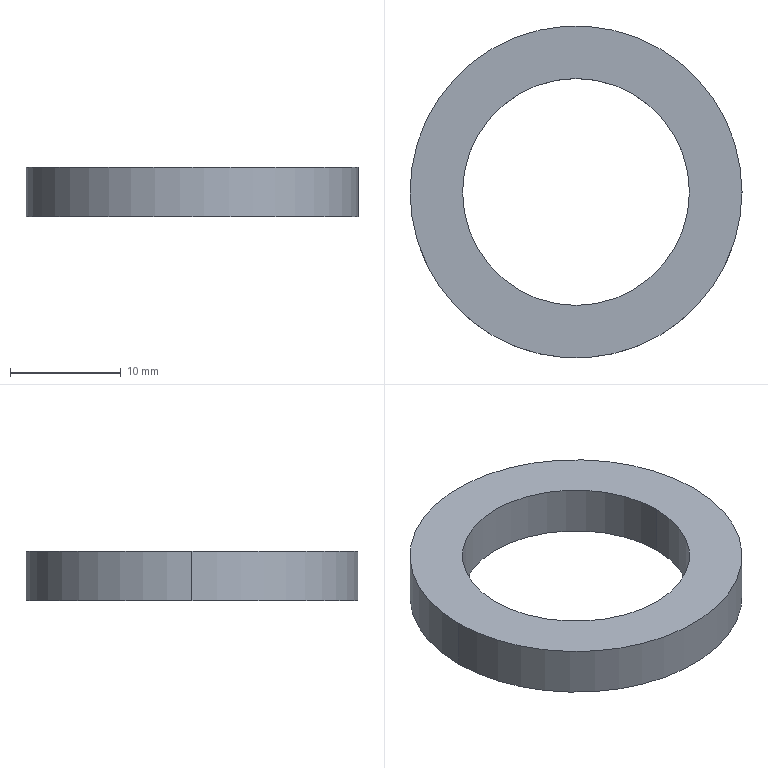Part | SolidWorks | features Extrusion 1 | 1 solid | 6 faces | box 30 x 30 x 4.5 mm | volume 1696 mm3 | cylinder 4 | plane 2 | commonest cylinder face diameters 20.5 x2 30 x2
STEP:
#1=CARTESIAN_POINT('',(-10.25,0.,4.5));
#2=VERTEX_POINT('',#1);
#3=CARTESIAN_POINT('',(10.25,0.,4.5));
#4=VERTEX_POINT('',#3);
#5=CARTESIAN_POINT('',(0.,0.,4.5));
#6=DIRECTION('',(0.,0.,1.));
#7=DIRECTION('',(1.,0.,0.));
#8=AXIS2_PLACEMENT_3D('',#5,#6,#7);
#9=CIRCLE('',#8,10.25);
#10=EDGE_CURVE('',#2,#4,#9,.T.);
#11=ORIENTED_EDGE('',*,*,#10,.T.);
#12=CARTESIAN_POINT('',(10.25,0.,0.));
#13=VERTEX_POINT('',#12);
#14=CARTESIAN_POINT('',(10.25,0.,4.5));
#15=DIRECTION('',(0.,0.,-1.));
#16=VECTOR('',#15,1000.);
#17=LINE('',#14,#16);
#18=EDGE_CURVE('',#4,#13,#17,.T.);
#19=ORIENTED_EDGE('',*,*,#18,.T.);
#20=CARTESIAN_POINT('',(-10.25,0.,0.));
#21=VERTEX_POINT('',#20);
#22=CARTESIAN_POINT('',(0.,0.,0.));
#23=DIRECTION('',(0.,0.,1.));
#24=DIRECTION('',(1.,0.,0.));
#25=AXIS2_PLACEMENT_3D('',#22,#23,#24);
#26=CIRCLE('',#25,10.25);
#27=EDGE_CURVE('',#21,#13,#26,.T.);
#28=ORIENTED_EDGE('',*,*,#27,.F.);
#29=CARTESIAN_POINT('',(-10.25,0.,4.5));
#30=DIRECTION('',(0.,0.,-1.));
#31=VECTOR('',#30,1000.);
#32=LINE('',#29,#31);
#33=EDGE_CURVE('',#2,#21,#32,.T.);
#34=ORIENTED_EDGE('',*,*,#33,.F.);
#35=EDGE_LOOP('',(#11,#19,#28,#34));
#36=FACE_OUTER_BOUND('',#35,.T.);
#37=CARTESIAN_POINT('',(0.,0.,4.5));
#38=DIRECTION('',(0.,0.,-1.));
#39=DIRECTION('',(-1.,0.,0.));
#40=AXIS2_PLACEMENT_3D('',#37,#38,#39);
#41=CYLINDRICAL_SURFACE('',#40,10.25);
#42=ADVANCED_FACE('',(#36),#41,.F.);
#43=CARTESIAN_POINT('',(15.,0.,4.5));
#44=VERTEX_POINT('',#43);
#45=CARTESIAN_POINT('',(-15.,0.,4.5));
#46=VERTEX_POINT('',#45);
#47=CARTESIAN_POINT('',(0.,0.,4.5));
#48=DIRECTION('',(0.,0.,1.));
#49=DIRECTION('',(1.,0.,0.));
#50=AXIS2_PLACEMENT_3D('',#47,#48,#49);
#51=CIRCLE('',#50,15.);
#52=EDGE_CURVE('',#44,#46,#51,.T.);
#53=ORIENTED_EDGE('',*,*,#52,.F.);
#54=CARTESIAN_POINT('',(15.,0.,0.));
#55=VERTEX_POINT('',#54);
#56=CARTESIAN_POINT('',(15.,0.,4.5));
#57=DIRECTION('',(0.,0.,-1.));
#58=VECTOR('',#57,1000.);
#59=LINE('',#56,#58);
#60=EDGE_CURVE('',#44,#55,#59,.T.);
#61=ORIENTED_EDGE('',*,*,#60,.T.);
#62=CARTESIAN_POINT('',(-15.,0.,0.));
#63=VERTEX_POINT('',#62);
#64=CARTESIAN_POINT('',(0.,0.,0.));
#65=DIRECTION('',(0.,0.,1.));
#66=DIRECTION('',(1.,0.,0.));
#67=AXIS2_PLACEMENT_3D('',#64,#65,#66);
#68=CIRCLE('',#67,15.);
#69=EDGE_CURVE('',#55,#63,#68,.T.);
#70=ORIENTED_EDGE('',*,*,#69,.T.);
#71=CARTESIAN_POINT('',(-15.,0.,4.5));
#72=DIRECTION('',(0.,0.,-1.));
#73=VECTOR('',#72,1000.);
#74=LINE('',#71,#73);
#75=EDGE_CURVE('',#46,#63,#74,.T.);
#76=ORIENTED_EDGE('',*,*,#75,.F.);
#77=EDGE_LOOP('',(#53,#61,#70,#76));
#78=FACE_OUTER_BOUND('',#77,.T.);
#79=CARTESIAN_POINT('',(0.,0.,4.5));
#80=DIRECTION('',(0.,0.,-1.));
#81=DIRECTION('',(-1.,0.,0.));
#82=AXIS2_PLACEMENT_3D('',#79,#80,#81);
#83=CYLINDRICAL_SURFACE('',#82,15.);
#84=ADVANCED_FACE('',(#78),#83,.T.);
#85=CARTESIAN_POINT('',(0.,0.,4.5));
#86=DIRECTION('',(0.,0.,1.));
#87=DIRECTION('',(1.,0.,0.));
#88=AXIS2_PLACEMENT_3D('',#85,#86,#87);
#89=CIRCLE('',#88,15.);
#90=EDGE_CURVE('',#46,#44,#89,.T.);
#91=ORIENTED_EDGE('',*,*,#90,.T.);
#92=ORIENTED_EDGE('',*,*,#52,.T.);
#93=EDGE_LOOP('',(#91,#92));
#94=FACE_OUTER_BOUND('',#93,.T.);
#95=ORIENTED_EDGE('',*,*,#10,.F.);
#96=CARTESIAN_POINT('',(0.,0.,4.5));
#97=DIRECTION('',(0.,0.,1.));
#98=DIRECTION('',(1.,0.,0.));
#99=AXIS2_PLACEMENT_3D('',#96,#97,#98);
#100=CIRCLE('',#99,10.25);
#101=EDGE_CURVE('',#4,#2,#100,.T.);
#102=ORIENTED_EDGE('',*,*,#101,.F.);
#103=EDGE_LOOP('',(#95,#102));
#104=FACE_BOUND('',#103,.T.);
#105=CARTESIAN_POINT('',(0.,0.,4.5));
#106=DIRECTION('',(0.,0.,1.));
#107=DIRECTION('',(1.,0.,0.));
#108=AXIS2_PLACEMENT_3D('',#105,#106,#107);
#109=PLANE('',#108);
#110=ADVANCED_FACE('',(#94,#104),#109,.T.);
#111=CARTESIAN_POINT('',(0.,0.,0.));
#112=DIRECTION('',(0.,0.,1.));
#113=DIRECTION('',(1.,0.,0.));
#114=AXIS2_PLACEMENT_3D('',#111,#112,#113);
#115=CIRCLE('',#114,15.);
#116=EDGE_CURVE('',#63,#55,#115,.T.);
#117=ORIENTED_EDGE('',*,*,#116,.F.);
#118=ORIENTED_EDGE('',*,*,#69,.F.);
#119=EDGE_LOOP('',(#117,#118));
#120=FACE_OUTER_BOUND('',#119,.T.);
#121=ORIENTED_EDGE('',*,*,#27,.T.);
#122=CARTESIAN_POINT('',(0.,0.,0.));
#123=DIRECTION('',(0.,0.,1.));
#124=DIRECTION('',(1.,0.,0.));
#125=AXIS2_PLACEMENT_3D('',#122,#123,#124);
#126=CIRCLE('',#125,10.25);
#127=EDGE_CURVE('',#13,#21,#126,.T.);
#128=ORIENTED_EDGE('',*,*,#127,.T.);
#129=EDGE_LOOP('',(#121,#128));
#130=FACE_BOUND('',#129,.T.);
#131=CARTESIAN_POINT('',(0.,0.,0.));
#132=DIRECTION('',(0.,0.,1.));
#133=DIRECTION('',(1.,0.,0.));
#134=AXIS2_PLACEMENT_3D('',#131,#132,#133);
#135=PLANE('',#134);
#136=ADVANCED_FACE('',(#120,#130),#135,.F.);
#137=ORIENTED_EDGE('',*,*,#60,.F.);
#138=ORIENTED_EDGE('',*,*,#90,.F.);
#139=ORIENTED_EDGE('',*,*,#75,.T.);
#140=ORIENTED_EDGE('',*,*,#116,.T.);
#141=EDGE_LOOP('',(#137,#138,#139,#140));
#142=FACE_OUTER_BOUND('',#141,.T.);
#143=CARTESIAN_POINT('',(0.,0.,4.5));
#144=DIRECTION('',(0.,0.,-1.));
#145=DIRECTION('',(-1.,0.,0.));
#146=AXIS2_PLACEMENT_3D('',#143,#144,#145);
#147=CYLINDRICAL_SURFACE('',#146,15.);
#148=ADVANCED_FACE('',(#142),#147,.T.);
#149=ORIENTED_EDGE('',*,*,#18,.F.);
#150=ORIENTED_EDGE('',*,*,#101,.T.);
#151=ORIENTED_EDGE('',*,*,#33,.T.);
#152=ORIENTED_EDGE('',*,*,#127,.F.);
#153=EDGE_LOOP('',(#149,#150,#151,#152));
#154=FACE_OUTER_BOUND('',#153,.T.);
#155=CARTESIAN_POINT('',(0.,0.,4.5));
#156=DIRECTION('',(0.,0.,-1.));
#157=DIRECTION('',(-1.,0.,0.));
#158=AXIS2_PLACEMENT_3D('',#155,#156,#157);
#159=CYLINDRICAL_SURFACE('',#158,10.25);
#160=ADVANCED_FACE('',(#154),#159,.F.);
#161=CLOSED_SHELL('',(#42,#84,#110,#136,#148,#160));
#162=MANIFOLD_SOLID_BREP('',#161);
#163=CARTESIAN_POINT('',(0.,0.,0.));
#164=DIRECTION('',(0.,0.,1.));
#165=DIRECTION('',(1.,0.,0.));
#166=AXIS2_PLACEMENT_3D('',#163,#164,#165);
#167=(LENGTH_UNIT()NAMED_UNIT(*)SI_UNIT(.MILLI.,.METRE.));
#168=UNCERTAINTY_MEASURE_WITH_UNIT(LENGTH_MEASURE(0.00001),#167,'','');
#169=(NAMED_UNIT(*)PLANE_ANGLE_UNIT()SI_UNIT($,.RADIAN.));
#170=(NAMED_UNIT(*)SI_UNIT($,.STERADIAN.)SOLID_ANGLE_UNIT());
#171=(GEOMETRIC_REPRESENTATION_CONTEXT(3)GLOBAL_UNCERTAINTY_ASSIGNED_CONTEXT((#168))GLOBAL_UNIT_ASSIGNED_CONTEXT((#167,#169,#170))REPRESENTATION_CONTEXT('',''));
#172=ADVANCED_BREP_SHAPE_REPRESENTATION('',(#162,#166),#171);